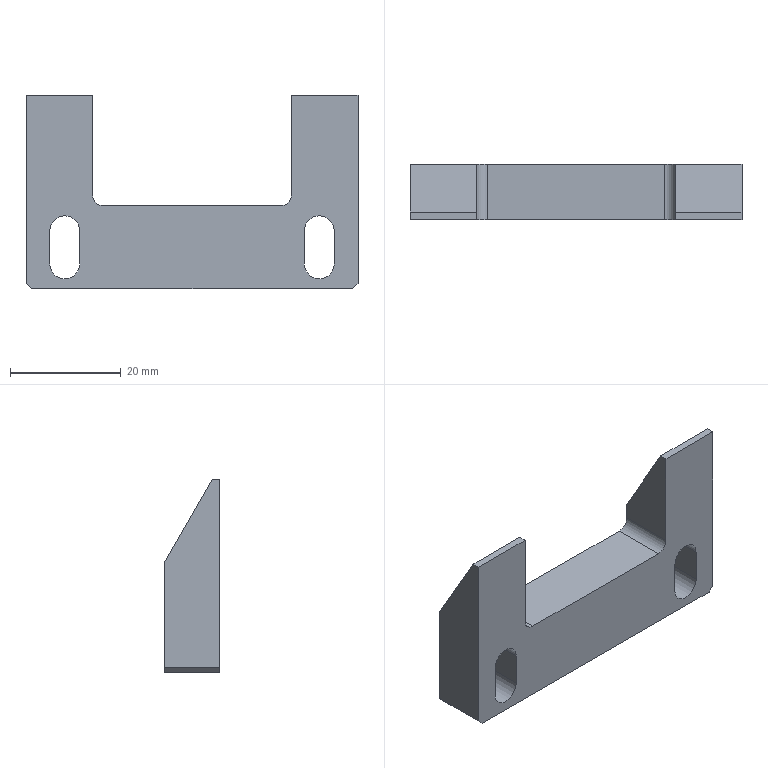Part | SolidWorks | features Chamfer 2, Cut 1, Extrusion 1, Fillet 1, ICE 1, MirrorPattern 1 | 1 solid | 26 faces | box 60 x 10 x 35 mm | volume 11142 mm3 | plane 18 | cylinder 8 | commonest cylinder face diameters 5.4 x6 4 x2
STEP:
#1=CARTESIAN_POINT('',(25.7,0.,-7.));
#2=VERTEX_POINT('',#1);
#3=CARTESIAN_POINT('',(23.,0.,-4.3));
#4=VERTEX_POINT('',#3);
#5=CARTESIAN_POINT('',(23.,0.,-7.));
#6=DIRECTION('',(0.,-1.,0.));
#7=DIRECTION('',(0.,0.,1.));
#8=AXIS2_PLACEMENT_3D('',#5,#6,#7);
#9=CIRCLE('',#8,2.7);
#10=EDGE_CURVE('',#2,#4,#9,.T.);
#11=ORIENTED_EDGE('',*,*,#10,.T.);
#12=CARTESIAN_POINT('',(23.,10.,-4.3));
#13=VERTEX_POINT('',#12);
#14=CARTESIAN_POINT('',(23.,0.,-4.3));
#15=DIRECTION('',(0.,1.,0.));
#16=VECTOR('',#15,1000.);
#17=LINE('',#14,#16);
#18=EDGE_CURVE('',#4,#13,#17,.T.);
#19=ORIENTED_EDGE('',*,*,#18,.T.);
#20=CARTESIAN_POINT('',(25.7,10.,-7.));
#21=VERTEX_POINT('',#20);
#22=CARTESIAN_POINT('',(23.,10.,-7.));
#23=DIRECTION('',(0.,-1.,0.));
#24=DIRECTION('',(0.,0.,1.));
#25=AXIS2_PLACEMENT_3D('',#22,#23,#24);
#26=CIRCLE('',#25,2.7);
#27=EDGE_CURVE('',#21,#13,#26,.T.);
#28=ORIENTED_EDGE('',*,*,#27,.F.);
#29=CARTESIAN_POINT('',(25.7,0.,-7.));
#30=DIRECTION('',(0.,1.,0.));
#31=VECTOR('',#30,1000.);
#32=LINE('',#29,#31);
#33=EDGE_CURVE('',#2,#21,#32,.T.);
#34=ORIENTED_EDGE('',*,*,#33,.F.);
#35=EDGE_LOOP('',(#11,#19,#28,#34));
#36=FACE_OUTER_BOUND('',#35,.T.);
#37=CARTESIAN_POINT('',(23.,0.,-7.));
#38=DIRECTION('',(0.,1.,0.));
#39=DIRECTION('',(0.,0.,1.));
#40=AXIS2_PLACEMENT_3D('',#37,#38,#39);
#41=CYLINDRICAL_SURFACE('',#40,2.7);
#42=ADVANCED_FACE('',(#36),#41,.F.);
#43=CARTESIAN_POINT('',(-23.,0.,-4.3));
#44=VERTEX_POINT('',#43);
#45=CARTESIAN_POINT('',(-20.3,0.,-7.));
#46=VERTEX_POINT('',#45);
#47=CARTESIAN_POINT('',(-23.,0.,-7.));
#48=DIRECTION('',(0.,1.,0.));
#49=DIRECTION('',(0.,0.,1.));
#50=AXIS2_PLACEMENT_3D('',#47,#48,#49);
#51=CIRCLE('',#50,2.7);
#52=EDGE_CURVE('',#44,#46,#51,.T.);
#53=ORIENTED_EDGE('',*,*,#52,.F.);
#54=CARTESIAN_POINT('',(-23.,10.,-4.3));
#55=VERTEX_POINT('',#54);
#56=CARTESIAN_POINT('',(-23.,0.,-4.3));
#57=DIRECTION('',(0.,1.,0.));
#58=VECTOR('',#57,1000.);
#59=LINE('',#56,#58);
#60=EDGE_CURVE('',#44,#55,#59,.T.);
#61=ORIENTED_EDGE('',*,*,#60,.T.);
#62=CARTESIAN_POINT('',(-20.3,10.,-7.));
#63=VERTEX_POINT('',#62);
#64=CARTESIAN_POINT('',(-23.,10.,-7.));
#65=DIRECTION('',(0.,1.,0.));
#66=DIRECTION('',(0.,0.,1.));
#67=AXIS2_PLACEMENT_3D('',#64,#65,#66);
#68=CIRCLE('',#67,2.7);
#69=EDGE_CURVE('',#55,#63,#68,.T.);
#70=ORIENTED_EDGE('',*,*,#69,.T.);
#71=CARTESIAN_POINT('',(-20.3,0.,-7.));
#72=DIRECTION('',(0.,1.,0.));
#73=VECTOR('',#72,1000.);
#74=LINE('',#71,#73);
#75=EDGE_CURVE('',#46,#63,#74,.T.);
#76=ORIENTED_EDGE('',*,*,#75,.F.);
#77=EDGE_LOOP('',(#53,#61,#70,#76));
#78=FACE_OUTER_BOUND('',#77,.T.);
#79=CARTESIAN_POINT('',(-23.,0.,-7.));
#80=DIRECTION('',(0.,1.,0.));
#81=DIRECTION('',(0.,0.,1.));
#82=AXIS2_PLACEMENT_3D('',#79,#80,#81);
#83=CYLINDRICAL_SURFACE('',#82,2.7);
#84=ADVANCED_FACE('',(#78),#83,.F.);
#85=CARTESIAN_POINT('',(30.,10.,2.5));
#86=VERTEX_POINT('',#85);
#87=CARTESIAN_POINT('',(30.,10.,-16.5));
#88=VERTEX_POINT('',#87);
#89=CARTESIAN_POINT('',(30.,10.,-17.5));
#90=DIRECTION('',(0.,0.,-1.));
#91=VECTOR('',#90,1000.);
#92=LINE('',#89,#91);
#93=EDGE_CURVE('',#86,#88,#92,.T.);
#94=ORIENTED_EDGE('',*,*,#93,.T.);
#95=CARTESIAN_POINT('',(29.,10.,-17.5));
#96=VERTEX_POINT('',#95);
#97=CARTESIAN_POINT('',(23.25,10.,-23.25));
#98=DIRECTION('',(-0.7071,0.,-0.7071));
#99=VECTOR('',#98,1000.);
#100=LINE('',#97,#99);
#101=EDGE_CURVE('',#88,#96,#100,.T.);
#102=ORIENTED_EDGE('',*,*,#101,.T.);
#103=CARTESIAN_POINT('',(-29.,10.,-17.5));
#104=VERTEX_POINT('',#103);
#105=CARTESIAN_POINT('',(-30.,10.,-17.5));
#106=DIRECTION('',(-1.,0.,0.));
#107=VECTOR('',#106,1000.);
#108=LINE('',#105,#107);
#109=EDGE_CURVE('',#96,#104,#108,.T.);
#110=ORIENTED_EDGE('',*,*,#109,.T.);
#111=CARTESIAN_POINT('',(-30.,10.,-16.5));
#112=VERTEX_POINT('',#111);
#113=CARTESIAN_POINT('',(-23.25,10.,-23.25));
#114=DIRECTION('',(-0.7071,0.,0.7071));
#115=VECTOR('',#114,1000.);
#116=LINE('',#113,#115);
#117=EDGE_CURVE('',#104,#112,#116,.T.);
#118=ORIENTED_EDGE('',*,*,#117,.T.);
#119=CARTESIAN_POINT('',(-30.,10.,2.5));
#120=VERTEX_POINT('',#119);
#121=CARTESIAN_POINT('',(-30.,10.,-17.5));
#122=DIRECTION('',(0.,0.,1.));
#123=VECTOR('',#122,1000.);
#124=LINE('',#121,#123);
#125=EDGE_CURVE('',#112,#120,#124,.T.);
#126=ORIENTED_EDGE('',*,*,#125,.T.);
#127=CARTESIAN_POINT('',(-18.,10.,2.5));
#128=VERTEX_POINT('',#127);
#129=CARTESIAN_POINT('',(30.,10.,2.5));
#130=DIRECTION('',(1.,0.,0.));
#131=VECTOR('',#130,1000.);
#132=LINE('',#129,#131);
#133=EDGE_CURVE('',#120,#128,#132,.T.);
#134=ORIENTED_EDGE('',*,*,#133,.T.);
#135=CARTESIAN_POINT('',(-18.,10.,-0.5));
#136=VERTEX_POINT('',#135);
#137=CARTESIAN_POINT('',(-18.,10.,17.5));
#138=DIRECTION('',(0.,0.,1.));
#139=VECTOR('',#138,1000.);
#140=LINE('',#137,#139);
#141=EDGE_CURVE('',#136,#128,#140,.T.);
#142=ORIENTED_EDGE('',*,*,#141,.F.);
#143=CARTESIAN_POINT('',(-16.,10.,-2.5));
#144=VERTEX_POINT('',#143);
#145=CARTESIAN_POINT('',(-16.,10.,-0.5));
#146=DIRECTION('',(0.,-1.,0.));
#147=DIRECTION('',(0.,0.,1.));
#148=AXIS2_PLACEMENT_3D('',#145,#146,#147);
#149=CIRCLE('',#148,2.);
#150=EDGE_CURVE('',#136,#144,#149,.T.);
#151=ORIENTED_EDGE('',*,*,#150,.T.);
#152=CARTESIAN_POINT('',(16.,10.,-2.5));
#153=VERTEX_POINT('',#152);
#154=CARTESIAN_POINT('',(-18.,10.,-2.5));
#155=DIRECTION('',(-1.,0.,0.));
#156=VECTOR('',#155,1000.);
#157=LINE('',#154,#156);
#158=EDGE_CURVE('',#153,#144,#157,.T.);
#159=ORIENTED_EDGE('',*,*,#158,.F.);
#160=CARTESIAN_POINT('',(18.,10.,-0.5));
#161=VERTEX_POINT('',#160);
#162=CARTESIAN_POINT('',(16.,10.,-0.5));
#163=DIRECTION('',(0.,-1.,0.));
#164=DIRECTION('',(0.,0.,1.));
#165=AXIS2_PLACEMENT_3D('',#162,#163,#164);
#166=CIRCLE('',#165,2.);
#167=EDGE_CURVE('',#153,#161,#166,.T.);
#168=ORIENTED_EDGE('',*,*,#167,.T.);
#169=CARTESIAN_POINT('',(18.,10.,2.5));
#170=VERTEX_POINT('',#169);
#171=CARTESIAN_POINT('',(18.,10.,17.5));
#172=DIRECTION('',(0.,0.,-1.));
#173=VECTOR('',#172,1000.);
#174=LINE('',#171,#173);
#175=EDGE_CURVE('',#170,#161,#174,.T.);
#176=ORIENTED_EDGE('',*,*,#175,.F.);
#177=CARTESIAN_POINT('',(30.,10.,2.5));
#178=DIRECTION('',(1.,0.,0.));
#179=VECTOR('',#178,1000.);
#180=LINE('',#177,#179);
#181=EDGE_CURVE('',#170,#86,#180,.T.);
#182=ORIENTED_EDGE('',*,*,#181,.T.);
#183=EDGE_LOOP('',(#94,#102,#110,#118,#126,#134,#142,#151,#159,#168,#176,#182));
#184=FACE_OUTER_BOUND('',#183,.T.);
#185=CARTESIAN_POINT('',(-20.3,10.,-13.));
#186=VERTEX_POINT('',#185);
#187=CARTESIAN_POINT('',(-25.7,10.,-13.));
#188=VERTEX_POINT('',#187);
#189=CARTESIAN_POINT('',(-23.,10.,-13.));
#190=DIRECTION('',(0.,1.,0.));
#191=DIRECTION('',(0.,0.,1.));
#192=AXIS2_PLACEMENT_3D('',#189,#190,#191);
#193=CIRCLE('',#192,2.7);
#194=EDGE_CURVE('',#186,#188,#193,.T.);
#195=ORIENTED_EDGE('',*,*,#194,.F.);
#196=CARTESIAN_POINT('',(-20.3,10.,-13.));
#197=DIRECTION('',(0.,0.,-1.));
#198=VECTOR('',#197,1000.);
#199=LINE('',#196,#198);
#200=EDGE_CURVE('',#63,#186,#199,.T.);
#201=ORIENTED_EDGE('',*,*,#200,.F.);
#202=ORIENTED_EDGE('',*,*,#69,.F.);
#203=CARTESIAN_POINT('',(-25.7,10.,-7.));
#204=VERTEX_POINT('',#203);
#205=CARTESIAN_POINT('',(-23.,10.,-7.));
#206=DIRECTION('',(0.,1.,0.));
#207=DIRECTION('',(0.,0.,1.));
#208=AXIS2_PLACEMENT_3D('',#205,#206,#207);
#209=CIRCLE('',#208,2.7);
#210=EDGE_CURVE('',#204,#55,#209,.T.);
#211=ORIENTED_EDGE('',*,*,#210,.F.);
#212=CARTESIAN_POINT('',(-25.7,10.,-13.));
#213=DIRECTION('',(0.,0.,1.));
#214=VECTOR('',#213,1000.);
#215=LINE('',#212,#214);
#216=EDGE_CURVE('',#188,#204,#215,.T.);
#217=ORIENTED_EDGE('',*,*,#216,.F.);
#218=EDGE_LOOP('',(#195,#201,#202,#211,#217));
#219=FACE_BOUND('',#218,.T.);
#220=CARTESIAN_POINT('',(20.3,10.,-7.));
#221=VERTEX_POINT('',#220);
#222=CARTESIAN_POINT('',(20.3,10.,-13.));
#223=VERTEX_POINT('',#222);
#224=CARTESIAN_POINT('',(20.3,10.,-13.));
#225=DIRECTION('',(0.,0.,-1.));
#226=VECTOR('',#225,1000.);
#227=LINE('',#224,#226);
#228=EDGE_CURVE('',#221,#223,#227,.T.);
#229=ORIENTED_EDGE('',*,*,#228,.T.);
#230=CARTESIAN_POINT('',(25.7,10.,-13.));
#231=VERTEX_POINT('',#230);
#232=CARTESIAN_POINT('',(23.,10.,-13.));
#233=DIRECTION('',(0.,-1.,0.));
#234=DIRECTION('',(0.,0.,1.));
#235=AXIS2_PLACEMENT_3D('',#232,#233,#234);
#236=CIRCLE('',#235,2.7);
#237=EDGE_CURVE('',#223,#231,#236,.T.);
#238=ORIENTED_EDGE('',*,*,#237,.T.);
#239=CARTESIAN_POINT('',(25.7,10.,-13.));
#240=DIRECTION('',(0.,0.,1.));
#241=VECTOR('',#240,1000.);
#242=LINE('',#239,#241);
#243=EDGE_CURVE('',#231,#21,#242,.T.);
#244=ORIENTED_EDGE('',*,*,#243,.T.);
#245=ORIENTED_EDGE('',*,*,#27,.T.);
#246=CARTESIAN_POINT('',(23.,10.,-7.));
#247=DIRECTION('',(0.,-1.,0.));
#248=DIRECTION('',(0.,0.,1.));
#249=AXIS2_PLACEMENT_3D('',#246,#247,#248);
#250=CIRCLE('',#249,2.7);
#251=EDGE_CURVE('',#13,#221,#250,.T.);
#252=ORIENTED_EDGE('',*,*,#251,.T.);
#253=EDGE_LOOP('',(#229,#238,#244,#245,#252));
#254=FACE_BOUND('',#253,.T.);
#255=CARTESIAN_POINT('',(0.,10.,0.));
#256=DIRECTION('',(0.,1.,0.));
#257=DIRECTION('',(0.,0.,1.));
#258=AXIS2_PLACEMENT_3D('',#255,#256,#257);
#259=PLANE('',#258);
#260=ADVANCED_FACE('',(#184,#219,#254),#259,.T.);
#261=CARTESIAN_POINT('',(29.,0.,-17.5));
#262=VERTEX_POINT('',#261);
#263=CARTESIAN_POINT('',(-29.,0.,-17.5));
#264=VERTEX_POINT('',#263);
#265=CARTESIAN_POINT('',(-30.,0.,-17.5));
#266=DIRECTION('',(-1.,0.,0.));
#267=VECTOR('',#266,1000.);
#268=LINE('',#265,#267);
#269=EDGE_CURVE('',#262,#264,#268,.T.);
#270=ORIENTED_EDGE('',*,*,#269,.F.);
#271=CARTESIAN_POINT('',(30.,0.,-16.5));
#272=VERTEX_POINT('',#271);
#273=CARTESIAN_POINT('',(29.,0.,-17.5));
#274=DIRECTION('',(0.7071,0.,0.7071));
#275=VECTOR('',#274,1000.);
#276=LINE('',#273,#275);
#277=EDGE_CURVE('',#262,#272,#276,.T.);
#278=ORIENTED_EDGE('',*,*,#277,.T.);
#279=CARTESIAN_POINT('',(30.,0.,17.5));
#280=VERTEX_POINT('',#279);
#281=CARTESIAN_POINT('',(30.,0.,-17.5));
#282=DIRECTION('',(0.,0.,-1.));
#283=VECTOR('',#282,1000.);
#284=LINE('',#281,#283);
#285=EDGE_CURVE('',#280,#272,#284,.T.);
#286=ORIENTED_EDGE('',*,*,#285,.F.);
#287=CARTESIAN_POINT('',(18.,0.,17.5));
#288=VERTEX_POINT('',#287);
#289=CARTESIAN_POINT('',(-30.,0.,17.5));
#290=DIRECTION('',(1.,0.,0.));
#291=VECTOR('',#290,1000.);
#292=LINE('',#289,#291);
#293=EDGE_CURVE('',#288,#280,#292,.T.);
#294=ORIENTED_EDGE('',*,*,#293,.F.);
#295=CARTESIAN_POINT('',(18.,0.,-0.5));
#296=VERTEX_POINT('',#295);
#297=CARTESIAN_POINT('',(18.,0.,17.5));
#298=DIRECTION('',(0.,0.,-1.));
#299=VECTOR('',#298,1000.);
#300=LINE('',#297,#299);
#301=EDGE_CURVE('',#288,#296,#300,.T.);
#302=ORIENTED_EDGE('',*,*,#301,.T.);
#303=CARTESIAN_POINT('',(16.,0.,-2.5));
#304=VERTEX_POINT('',#303);
#305=CARTESIAN_POINT('',(16.,0.,-0.5));
#306=DIRECTION('',(0.,1.,0.));
#307=DIRECTION('',(0.,0.,1.));
#308=AXIS2_PLACEMENT_3D('',#305,#306,#307);
#309=CIRCLE('',#308,2.);
#310=EDGE_CURVE('',#296,#304,#309,.T.);
#311=ORIENTED_EDGE('',*,*,#310,.T.);
#312=CARTESIAN_POINT('',(-16.,0.,-2.5));
#313=VERTEX_POINT('',#312);
#314=CARTESIAN_POINT('',(-18.,0.,-2.5));
#315=DIRECTION('',(-1.,0.,0.));
#316=VECTOR('',#315,1000.);
#317=LINE('',#314,#316);
#318=EDGE_CURVE('',#304,#313,#317,.T.);
#319=ORIENTED_EDGE('',*,*,#318,.T.);
#320=CARTESIAN_POINT('',(-18.,0.,-0.5));
#321=VERTEX_POINT('',#320);
#322=CARTESIAN_POINT('',(-16.,0.,-0.5));
#323=DIRECTION('',(0.,1.,0.));
#324=DIRECTION('',(0.,0.,1.));
#325=AXIS2_PLACEMENT_3D('',#322,#323,#324);
#326=CIRCLE('',#325,2.);
#327=EDGE_CURVE('',#313,#321,#326,.T.);
#328=ORIENTED_EDGE('',*,*,#327,.T.);
#329=CARTESIAN_POINT('',(-18.,0.,17.5));
#330=VERTEX_POINT('',#329);
#331=CARTESIAN_POINT('',(-18.,0.,17.5));
#332=DIRECTION('',(0.,0.,1.));
#333=VECTOR('',#332,1000.);
#334=LINE('',#331,#333);
#335=EDGE_CURVE('',#321,#330,#334,.T.);
#336=ORIENTED_EDGE('',*,*,#335,.T.);
#337=CARTESIAN_POINT('',(-30.,0.,17.5));
#338=VERTEX_POINT('',#337);
#339=CARTESIAN_POINT('',(-30.,0.,17.5));
#340=DIRECTION('',(1.,0.,0.));
#341=VECTOR('',#340,1000.);
#342=LINE('',#339,#341);
#343=EDGE_CURVE('',#338,#330,#342,.T.);
#344=ORIENTED_EDGE('',*,*,#343,.F.);
#345=CARTESIAN_POINT('',(-30.,0.,-16.5));
#346=VERTEX_POINT('',#345);
#347=CARTESIAN_POINT('',(-30.,0.,-17.5));
#348=DIRECTION('',(0.,0.,1.));
#349=VECTOR('',#348,1000.);
#350=LINE('',#347,#349);
#351=EDGE_CURVE('',#346,#338,#350,.T.);
#352=ORIENTED_EDGE('',*,*,#351,.F.);
#353=CARTESIAN_POINT('',(-30.,0.,-16.5));
#354=DIRECTION('',(0.7071,0.,-0.7071));
#355=VECTOR('',#354,1000.);
#356=LINE('',#353,#355);
#357=EDGE_CURVE('',#346,#264,#356,.T.);
#358=ORIENTED_EDGE('',*,*,#357,.T.);
#359=EDGE_LOOP('',(#270,#278,#286,#294,#302,#311,#319,#328,#336,#344,#352,#358));
#360=FACE_OUTER_BOUND('',#359,.T.);
#361=CARTESIAN_POINT('',(-20.3,0.,-13.));
#362=VERTEX_POINT('',#361);
#363=CARTESIAN_POINT('',(-20.3,0.,-13.));
#364=DIRECTION('',(0.,0.,-1.));
#365=VECTOR('',#364,1000.);
#366=LINE('',#363,#365);
#367=EDGE_CURVE('',#46,#362,#366,.T.);
#368=ORIENTED_EDGE('',*,*,#367,.T.);
#369=CARTESIAN_POINT('',(-25.7,0.,-13.));
#370=VERTEX_POINT('',#369);
#371=CARTESIAN_POINT('',(-23.,0.,-13.));
#372=DIRECTION('',(0.,1.,0.));
#373=DIRECTION('',(0.,0.,1.));
#374=AXIS2_PLACEMENT_3D('',#371,#372,#373);
#375=CIRCLE('',#374,2.7);
#376=EDGE_CURVE('',#362,#370,#375,.T.);
#377=ORIENTED_EDGE('',*,*,#376,.T.);
#378=CARTESIAN_POINT('',(-25.7,0.,-7.));
#379=VERTEX_POINT('',#378);
#380=CARTESIAN_POINT('',(-25.7,0.,-13.));
#381=DIRECTION('',(0.,0.,1.));
#382=VECTOR('',#381,1000.);
#383=LINE('',#380,#382);
#384=EDGE_CURVE('',#370,#379,#383,.T.);
#385=ORIENTED_EDGE('',*,*,#384,.T.);
#386=CARTESIAN_POINT('',(-23.,0.,-7.));
#387=DIRECTION('',(0.,1.,0.));
#388=DIRECTION('',(0.,0.,1.));
#389=AXIS2_PLACEMENT_3D('',#386,#387,#388);
#390=CIRCLE('',#389,2.7);
#391=EDGE_CURVE('',#379,#44,#390,.T.);
#392=ORIENTED_EDGE('',*,*,#391,.T.);
#393=ORIENTED_EDGE('',*,*,#52,.T.);
#394=EDGE_LOOP('',(#368,#377,#385,#392,#393));
#395=FACE_BOUND('',#394,.T.);
#396=CARTESIAN_POINT('',(20.3,0.,-13.));
#397=VERTEX_POINT('',#396);
#398=CARTESIAN_POINT('',(25.7,0.,-13.));
#399=VERTEX_POINT('',#398);
#400=CARTESIAN_POINT('',(23.,0.,-13.));
#401=DIRECTION('',(0.,-1.,0.));
#402=DIRECTION('',(0.,0.,1.));
#403=AXIS2_PLACEMENT_3D('',#400,#401,#402);
#404=CIRCLE('',#403,2.7);
#405=EDGE_CURVE('',#397,#399,#404,.T.);
#406=ORIENTED_EDGE('',*,*,#405,.F.);
#407=CARTESIAN_POINT('',(20.3,0.,-7.));
#408=VERTEX_POINT('',#407);
#409=CARTESIAN_POINT('',(20.3,0.,-13.));
#410=DIRECTION('',(0.,0.,-1.));
#411=VECTOR('',#410,1000.);
#412=LINE('',#409,#411);
#413=EDGE_CURVE('',#408,#397,#412,.T.);
#414=ORIENTED_EDGE('',*,*,#413,.F.);
#415=CARTESIAN_POINT('',(23.,0.,-7.));
#416=DIRECTION('',(0.,-1.,0.));
#417=DIRECTION('',(0.,0.,1.));
#418=AXIS2_PLACEMENT_3D('',#415,#416,#417);
#419=CIRCLE('',#418,2.7);
#420=EDGE_CURVE('',#4,#408,#419,.T.);
#421=ORIENTED_EDGE('',*,*,#420,.F.);
#422=ORIENTED_EDGE('',*,*,#10,.F.);
#423=CARTESIAN_POINT('',(25.7,0.,-13.));
#424=DIRECTION('',(0.,0.,1.));
#425=VECTOR('',#424,1000.);
#426=LINE('',#423,#425);
#427=EDGE_CURVE('',#399,#2,#426,.T.);
#428=ORIENTED_EDGE('',*,*,#427,.F.);
#429=EDGE_LOOP('',(#406,#414,#421,#422,#428));
#430=FACE_BOUND('',#429,.T.);
#431=CARTESIAN_POINT('',(0.,0.,0.));
#432=DIRECTION('',(0.,1.,0.));
#433=DIRECTION('',(0.,0.,1.));
#434=AXIS2_PLACEMENT_3D('',#431,#432,#433);
#435=PLANE('',#434);
#436=ADVANCED_FACE('',(#360,#395,#430),#435,.F.);
#437=ORIENTED_EDGE('',*,*,#343,.T.);
#438=CARTESIAN_POINT('',(-18.,1.34,17.5));
#439=VERTEX_POINT('',#438);
#440=CARTESIAN_POINT('',(-18.,0.,17.5));
#441=DIRECTION('',(0.,1.,0.));
#442=VECTOR('',#441,1000.);
#443=LINE('',#440,#442);
#444=EDGE_CURVE('',#330,#439,#443,.T.);
#445=ORIENTED_EDGE('',*,*,#444,.T.);
#446=CARTESIAN_POINT('',(-30.,1.34,17.5));
#447=VERTEX_POINT('',#446);
#448=CARTESIAN_POINT('',(-30.,1.34,17.5));
#449=DIRECTION('',(-1.,0.,0.));
#450=VECTOR('',#449,1000.);
#451=LINE('',#448,#450);
#452=EDGE_CURVE('',#439,#447,#451,.T.);
#453=ORIENTED_EDGE('',*,*,#452,.T.);
#454=CARTESIAN_POINT('',(-30.,10.,17.5));
#455=DIRECTION('',(0.,-1.,0.));
#456=VECTOR('',#455,1000.);
#457=LINE('',#454,#456);
#458=EDGE_CURVE('',#447,#338,#457,.T.);
#459=ORIENTED_EDGE('',*,*,#458,.T.);
#460=EDGE_LOOP('',(#437,#445,#453,#459));
#461=FACE_OUTER_BOUND('',#460,.T.);
#462=CARTESIAN_POINT('',(-30.,10.,17.5));
#463=DIRECTION('',(0.,0.,-1.));
#464=DIRECTION('',(-1.,0.,0.));
#465=AXIS2_PLACEMENT_3D('',#462,#463,#464);
#466=PLANE('',#465);
#467=ADVANCED_FACE('',(#461),#466,.F.);
#468=CARTESIAN_POINT('',(-18.,10.,2.5));
#469=DIRECTION('',(0.,-0.5,0.866));
#470=VECTOR('',#469,1000.);
#471=LINE('',#468,#470);
#472=EDGE_CURVE('',#128,#439,#471,.T.);
#473=ORIENTED_EDGE('',*,*,#472,.F.);
#474=ORIENTED_EDGE('',*,*,#133,.F.);
#475=CARTESIAN_POINT('',(-30.,10.,2.5));
#476=DIRECTION('',(0.,0.5,-0.866));
#477=VECTOR('',#476,1000.);
#478=LINE('',#475,#477);
#479=EDGE_CURVE('',#447,#120,#478,.T.);
#480=ORIENTED_EDGE('',*,*,#479,.F.);
#481=ORIENTED_EDGE('',*,*,#452,.F.);
#482=EDGE_LOOP('',(#473,#474,#480,#481));
#483=FACE_OUTER_BOUND('',#482,.T.);
#484=CARTESIAN_POINT('',(0.,10.,2.5));
#485=DIRECTION('',(0.,0.866,0.5));
#486=DIRECTION('',(-1.,0.,0.));
#487=AXIS2_PLACEMENT_3D('',#484,#485,#486);
#488=PLANE('',#487);
#489=ADVANCED_FACE('',(#483),#488,.T.);
#490=ORIENTED_EDGE('',*,*,#285,.T.);
#491=CARTESIAN_POINT('',(30.,10.,-16.5));
#492=DIRECTION('',(0.,1.,0.));
#493=VECTOR('',#492,1000.);
#494=LINE('',#491,#493);
#495=EDGE_CURVE('',#272,#88,#494,.T.);
#496=ORIENTED_EDGE('',*,*,#495,.T.);
#497=ORIENTED_EDGE('',*,*,#93,.F.);
#498=CARTESIAN_POINT('',(30.,1.34,17.5));
#499=VERTEX_POINT('',#498);
#500=CARTESIAN_POINT('',(30.,10.,2.5));
#501=DIRECTION('',(0.,-0.5,0.866));
#502=VECTOR('',#501,1000.);
#503=LINE('',#500,#502);
#504=EDGE_CURVE('',#86,#499,#503,.T.);
#505=ORIENTED_EDGE('',*,*,#504,.T.);
#506=CARTESIAN_POINT('',(30.,10.,17.5));
#507=DIRECTION('',(0.,-1.,0.));
#508=VECTOR('',#507,1000.);
#509=LINE('',#506,#508);
#510=EDGE_CURVE('',#499,#280,#509,.T.);
#511=ORIENTED_EDGE('',*,*,#510,.T.);
#512=EDGE_LOOP('',(#490,#496,#497,#505,#511));
#513=FACE_OUTER_BOUND('',#512,.T.);
#514=CARTESIAN_POINT('',(30.,10.,-17.5));
#515=DIRECTION('',(-1.,0.,0.));
#516=DIRECTION('',(0.,0.,1.));
#517=AXIS2_PLACEMENT_3D('',#514,#515,#516);
#518=PLANE('',#517);
#519=ADVANCED_FACE('',(#513),#518,.F.);
#520=ORIENTED_EDGE('',*,*,#109,.F.);
#521=CARTESIAN_POINT('',(29.,10.,-17.5));
#522=DIRECTION('',(0.,-1.,0.));
#523=VECTOR('',#522,1000.);
#524=LINE('',#521,#523);
#525=EDGE_CURVE('',#96,#262,#524,.T.);
#526=ORIENTED_EDGE('',*,*,#525,.T.);
#527=ORIENTED_EDGE('',*,*,#269,.T.);
#528=CARTESIAN_POINT('',(-29.,10.,-17.5));
#529=DIRECTION('',(0.,1.,0.));
#530=VECTOR('',#529,1000.);
#531=LINE('',#528,#530);
#532=EDGE_CURVE('',#264,#104,#531,.T.);
#533=ORIENTED_EDGE('',*,*,#532,.T.);
#534=EDGE_LOOP('',(#520,#526,#527,#533));
#535=FACE_OUTER_BOUND('',#534,.T.);
#536=CARTESIAN_POINT('',(-30.,10.,-17.5));
#537=DIRECTION('',(0.,0.,1.));
#538=DIRECTION('',(1.,0.,0.));
#539=AXIS2_PLACEMENT_3D('',#536,#537,#538);
#540=PLANE('',#539);
#541=ADVANCED_FACE('',(#535),#540,.F.);
#542=ORIENTED_EDGE('',*,*,#125,.F.);
#543=CARTESIAN_POINT('',(-30.,10.,-16.5));
#544=DIRECTION('',(0.,-1.,0.));
#545=VECTOR('',#544,1000.);
#546=LINE('',#543,#545);
#547=EDGE_CURVE('',#112,#346,#546,.T.);
#548=ORIENTED_EDGE('',*,*,#547,.T.);
#549=ORIENTED_EDGE('',*,*,#351,.T.);
#550=ORIENTED_EDGE('',*,*,#458,.F.);
#551=ORIENTED_EDGE('',*,*,#479,.T.);
#552=EDGE_LOOP('',(#542,#548,#549,#550,#551));
#553=FACE_OUTER_BOUND('',#552,.T.);
#554=CARTESIAN_POINT('',(-30.,10.,-17.5));
#555=DIRECTION('',(1.,0.,0.));
#556=DIRECTION('',(0.,0.,-1.));
#557=AXIS2_PLACEMENT_3D('',#554,#555,#556);
#558=PLANE('',#557);
#559=ADVANCED_FACE('',(#553),#558,.F.);
#560=CARTESIAN_POINT('',(18.,1.34,17.5));
#561=VERTEX_POINT('',#560);
#562=CARTESIAN_POINT('',(-30.,1.34,17.5));
#563=DIRECTION('',(-1.,0.,0.));
#564=VECTOR('',#563,1000.);
#565=LINE('',#562,#564);
#566=EDGE_CURVE('',#499,#561,#565,.T.);
#567=ORIENTED_EDGE('',*,*,#566,.T.);
#568=CARTESIAN_POINT('',(18.,0.,17.5));
#569=DIRECTION('',(0.,1.,0.));
#570=VECTOR('',#569,1000.);
#571=LINE('',#568,#570);
#572=EDGE_CURVE('',#288,#561,#571,.T.);
#573=ORIENTED_EDGE('',*,*,#572,.F.);
#574=ORIENTED_EDGE('',*,*,#293,.T.);
#575=ORIENTED_EDGE('',*,*,#510,.F.);
#576=EDGE_LOOP('',(#567,#573,#574,#575));
#577=FACE_OUTER_BOUND('',#576,.T.);
#578=CARTESIAN_POINT('',(-30.,10.,17.5));
#579=DIRECTION('',(0.,0.,-1.));
#580=DIRECTION('',(-1.,0.,0.));
#581=AXIS2_PLACEMENT_3D('',#578,#579,#580);
#582=PLANE('',#581);
#583=ADVANCED_FACE('',(#577),#582,.F.);
#584=CARTESIAN_POINT('',(18.,10.,2.5));
#585=DIRECTION('',(0.,0.5,-0.866));
#586=VECTOR('',#585,1000.);
#587=LINE('',#584,#586);
#588=EDGE_CURVE('',#561,#170,#587,.T.);
#589=ORIENTED_EDGE('',*,*,#588,.F.);
#590=ORIENTED_EDGE('',*,*,#566,.F.);
#591=ORIENTED_EDGE('',*,*,#504,.F.);
#592=ORIENTED_EDGE('',*,*,#181,.F.);
#593=EDGE_LOOP('',(#589,#590,#591,#592));
#594=FACE_OUTER_BOUND('',#593,.T.);
#595=CARTESIAN_POINT('',(0.,10.,2.5));
#596=DIRECTION('',(0.,0.866,0.5));
#597=DIRECTION('',(-1.,0.,0.));
#598=AXIS2_PLACEMENT_3D('',#595,#596,#597);
#599=PLANE('',#598);
#600=ADVANCED_FACE('',(#594),#599,.T.);
#601=ORIENTED_EDGE('',*,*,#335,.F.);
#602=CARTESIAN_POINT('',(-18.,10.,-0.5));
#603=DIRECTION('',(0.,1.,0.));
#604=VECTOR('',#603,1000.);
#605=LINE('',#602,#604);
#606=EDGE_CURVE('',#321,#136,#605,.T.);
#607=ORIENTED_EDGE('',*,*,#606,.T.);
#608=ORIENTED_EDGE('',*,*,#141,.T.);
#609=ORIENTED_EDGE('',*,*,#472,.T.);
#610=ORIENTED_EDGE('',*,*,#444,.F.);
#611=EDGE_LOOP('',(#601,#607,#608,#609,#610));
#612=FACE_OUTER_BOUND('',#611,.T.);
#613=CARTESIAN_POINT('',(-18.,0.,17.5));
#614=DIRECTION('',(-1.,0.,0.));
#615=DIRECTION('',(0.,0.,1.));
#616=AXIS2_PLACEMENT_3D('',#613,#614,#615);
#617=PLANE('',#616);
#618=ADVANCED_FACE('',(#612),#617,.F.);
#619=ORIENTED_EDGE('',*,*,#318,.F.);
#620=CARTESIAN_POINT('',(16.,10.,-2.5));
#621=DIRECTION('',(0.,1.,0.));
#622=VECTOR('',#621,1000.);
#623=LINE('',#620,#622);
#624=EDGE_CURVE('',#304,#153,#623,.T.);
#625=ORIENTED_EDGE('',*,*,#624,.T.);
#626=ORIENTED_EDGE('',*,*,#158,.T.);
#627=CARTESIAN_POINT('',(-16.,0.,-2.5));
#628=DIRECTION('',(0.,-1.,0.));
#629=VECTOR('',#628,1000.);
#630=LINE('',#627,#629);
#631=EDGE_CURVE('',#144,#313,#630,.T.);
#632=ORIENTED_EDGE('',*,*,#631,.T.);
#633=EDGE_LOOP('',(#619,#625,#626,#632));
#634=FACE_OUTER_BOUND('',#633,.T.);
#635=CARTESIAN_POINT('',(-18.,0.,-2.5));
#636=DIRECTION('',(0.,0.,-1.));
#637=DIRECTION('',(-1.,0.,0.));
#638=AXIS2_PLACEMENT_3D('',#635,#636,#637);
#639=PLANE('',#638);
#640=ADVANCED_FACE('',(#634),#639,.F.);
#641=ORIENTED_EDGE('',*,*,#175,.T.);
#642=CARTESIAN_POINT('',(18.,0.,-0.5));
#643=DIRECTION('',(0.,-1.,0.));
#644=VECTOR('',#643,1000.);
#645=LINE('',#642,#644);
#646=EDGE_CURVE('',#161,#296,#645,.T.);
#647=ORIENTED_EDGE('',*,*,#646,.T.);
#648=ORIENTED_EDGE('',*,*,#301,.F.);
#649=ORIENTED_EDGE('',*,*,#572,.T.);
#650=ORIENTED_EDGE('',*,*,#588,.T.);
#651=EDGE_LOOP('',(#641,#647,#648,#649,#650));
#652=FACE_OUTER_BOUND('',#651,.T.);
#653=CARTESIAN_POINT('',(18.,0.,17.5));
#654=DIRECTION('',(1.,0.,0.));
#655=DIRECTION('',(0.,0.,-1.));
#656=AXIS2_PLACEMENT_3D('',#653,#654,#655);
#657=PLANE('',#656);
#658=ADVANCED_FACE('',(#652),#657,.F.);
#659=ORIENTED_EDGE('',*,*,#310,.F.);
#660=ORIENTED_EDGE('',*,*,#646,.F.);
#661=ORIENTED_EDGE('',*,*,#167,.F.);
#662=ORIENTED_EDGE('',*,*,#624,.F.);
#663=EDGE_LOOP('',(#659,#660,#661,#662));
#664=FACE_OUTER_BOUND('',#663,.T.);
#665=CARTESIAN_POINT('',(16.,0.,-0.5));
#666=DIRECTION('',(0.,-1.,0.));
#667=DIRECTION('',(0.,0.,-1.));
#668=AXIS2_PLACEMENT_3D('',#665,#666,#667);
#669=CYLINDRICAL_SURFACE('',#668,2.);
#670=ADVANCED_FACE('',(#664),#669,.F.);
#671=ORIENTED_EDGE('',*,*,#327,.F.);
#672=ORIENTED_EDGE('',*,*,#631,.F.);
#673=ORIENTED_EDGE('',*,*,#150,.F.);
#674=ORIENTED_EDGE('',*,*,#606,.F.);
#675=EDGE_LOOP('',(#671,#672,#673,#674));
#676=FACE_OUTER_BOUND('',#675,.T.);
#677=CARTESIAN_POINT('',(-16.,0.,-0.5));
#678=DIRECTION('',(0.,-1.,0.));
#679=DIRECTION('',(0.,0.,-1.));
#680=AXIS2_PLACEMENT_3D('',#677,#678,#679);
#681=CYLINDRICAL_SURFACE('',#680,2.);
#682=ADVANCED_FACE('',(#676),#681,.F.);
#683=ORIENTED_EDGE('',*,*,#194,.T.);
#684=CARTESIAN_POINT('',(-25.7,0.,-13.));
#685=DIRECTION('',(0.,1.,0.));
#686=VECTOR('',#685,1000.);
#687=LINE('',#684,#686);
#688=EDGE_CURVE('',#370,#188,#687,.T.);
#689=ORIENTED_EDGE('',*,*,#688,.F.);
#690=ORIENTED_EDGE('',*,*,#376,.F.);
#691=CARTESIAN_POINT('',(-20.3,0.,-13.));
#692=DIRECTION('',(0.,1.,0.));
#693=VECTOR('',#692,1000.);
#694=LINE('',#691,#693);
#695=EDGE_CURVE('',#362,#186,#694,.T.);
#696=ORIENTED_EDGE('',*,*,#695,.T.);
#697=EDGE_LOOP('',(#683,#689,#690,#696));
#698=FACE_OUTER_BOUND('',#697,.T.);
#699=CARTESIAN_POINT('',(-23.,0.,-13.));
#700=DIRECTION('',(0.,1.,0.));
#701=DIRECTION('',(0.,0.,1.));
#702=AXIS2_PLACEMENT_3D('',#699,#700,#701);
#703=CYLINDRICAL_SURFACE('',#702,2.7);
#704=ADVANCED_FACE('',(#698),#703,.F.);
#705=ORIENTED_EDGE('',*,*,#200,.T.);
#706=ORIENTED_EDGE('',*,*,#695,.F.);
#707=ORIENTED_EDGE('',*,*,#367,.F.);
#708=ORIENTED_EDGE('',*,*,#75,.T.);
#709=EDGE_LOOP('',(#705,#706,#707,#708));
#710=FACE_OUTER_BOUND('',#709,.T.);
#711=CARTESIAN_POINT('',(-20.3,0.,-13.));
#712=DIRECTION('',(1.,0.,0.));
#713=DIRECTION('',(0.,0.,-1.));
#714=AXIS2_PLACEMENT_3D('',#711,#712,#713);
#715=PLANE('',#714);
#716=ADVANCED_FACE('',(#710),#715,.F.);
#717=ORIENTED_EDGE('',*,*,#60,.F.);
#718=ORIENTED_EDGE('',*,*,#391,.F.);
#719=CARTESIAN_POINT('',(-25.7,0.,-7.));
#720=DIRECTION('',(0.,1.,0.));
#721=VECTOR('',#720,1000.);
#722=LINE('',#719,#721);
#723=EDGE_CURVE('',#379,#204,#722,.T.);
#724=ORIENTED_EDGE('',*,*,#723,.T.);
#725=ORIENTED_EDGE('',*,*,#210,.T.);
#726=EDGE_LOOP('',(#717,#718,#724,#725));
#727=FACE_OUTER_BOUND('',#726,.T.);
#728=CARTESIAN_POINT('',(-23.,0.,-7.));
#729=DIRECTION('',(0.,1.,0.));
#730=DIRECTION('',(0.,0.,1.));
#731=AXIS2_PLACEMENT_3D('',#728,#729,#730);
#732=CYLINDRICAL_SURFACE('',#731,2.7);
#733=ADVANCED_FACE('',(#727),#732,.F.);
#734=ORIENTED_EDGE('',*,*,#216,.T.);
#735=ORIENTED_EDGE('',*,*,#723,.F.);
#736=ORIENTED_EDGE('',*,*,#384,.F.);
#737=ORIENTED_EDGE('',*,*,#688,.T.);
#738=EDGE_LOOP('',(#734,#735,#736,#737));
#739=FACE_OUTER_BOUND('',#738,.T.);
#740=CARTESIAN_POINT('',(-25.7,0.,-13.));
#741=DIRECTION('',(-1.,0.,0.));
#742=DIRECTION('',(0.,0.,1.));
#743=AXIS2_PLACEMENT_3D('',#740,#741,#742);
#744=PLANE('',#743);
#745=ADVANCED_FACE('',(#739),#744,.F.);
#746=ORIENTED_EDGE('',*,*,#237,.F.);
#747=CARTESIAN_POINT('',(20.3,0.,-13.));
#748=DIRECTION('',(0.,1.,0.));
#749=VECTOR('',#748,1000.);
#750=LINE('',#747,#749);
#751=EDGE_CURVE('',#397,#223,#750,.T.);
#752=ORIENTED_EDGE('',*,*,#751,.F.);
#753=ORIENTED_EDGE('',*,*,#405,.T.);
#754=CARTESIAN_POINT('',(25.7,0.,-13.));
#755=DIRECTION('',(0.,1.,0.));
#756=VECTOR('',#755,1000.);
#757=LINE('',#754,#756);
#758=EDGE_CURVE('',#399,#231,#757,.T.);
#759=ORIENTED_EDGE('',*,*,#758,.T.);
#760=EDGE_LOOP('',(#746,#752,#753,#759));
#761=FACE_OUTER_BOUND('',#760,.T.);
#762=CARTESIAN_POINT('',(23.,0.,-13.));
#763=DIRECTION('',(0.,1.,0.));
#764=DIRECTION('',(0.,0.,1.));
#765=AXIS2_PLACEMENT_3D('',#762,#763,#764);
#766=CYLINDRICAL_SURFACE('',#765,2.7);
#767=ADVANCED_FACE('',(#761),#766,.F.);
#768=ORIENTED_EDGE('',*,*,#243,.F.);
#769=ORIENTED_EDGE('',*,*,#758,.F.);
#770=ORIENTED_EDGE('',*,*,#427,.T.);
#771=ORIENTED_EDGE('',*,*,#33,.T.);
#772=EDGE_LOOP('',(#768,#769,#770,#771));
#773=FACE_OUTER_BOUND('',#772,.T.);
#774=CARTESIAN_POINT('',(25.7,0.,-13.));
#775=DIRECTION('',(-1.,0.,0.));
#776=DIRECTION('',(0.,0.,1.));
#777=AXIS2_PLACEMENT_3D('',#774,#775,#776);
#778=PLANE('',#777);
#779=ADVANCED_FACE('',(#773),#778,.T.);
#780=ORIENTED_EDGE('',*,*,#18,.F.);
#781=ORIENTED_EDGE('',*,*,#420,.T.);
#782=CARTESIAN_POINT('',(20.3,0.,-7.));
#783=DIRECTION('',(0.,1.,0.));
#784=VECTOR('',#783,1000.);
#785=LINE('',#782,#784);
#786=EDGE_CURVE('',#408,#221,#785,.T.);
#787=ORIENTED_EDGE('',*,*,#786,.T.);
#788=ORIENTED_EDGE('',*,*,#251,.F.);
#789=EDGE_LOOP('',(#780,#781,#787,#788));
#790=FACE_OUTER_BOUND('',#789,.T.);
#791=CARTESIAN_POINT('',(23.,0.,-7.));
#792=DIRECTION('',(0.,1.,0.));
#793=DIRECTION('',(0.,0.,1.));
#794=AXIS2_PLACEMENT_3D('',#791,#792,#793);
#795=CYLINDRICAL_SURFACE('',#794,2.7);
#796=ADVANCED_FACE('',(#790),#795,.F.);
#797=ORIENTED_EDGE('',*,*,#228,.F.);
#798=ORIENTED_EDGE('',*,*,#786,.F.);
#799=ORIENTED_EDGE('',*,*,#413,.T.);
#800=ORIENTED_EDGE('',*,*,#751,.T.);
#801=EDGE_LOOP('',(#797,#798,#799,#800));
#802=FACE_OUTER_BOUND('',#801,.T.);
#803=CARTESIAN_POINT('',(20.3,0.,-13.));
#804=DIRECTION('',(1.,0.,0.));
#805=DIRECTION('',(0.,0.,-1.));
#806=AXIS2_PLACEMENT_3D('',#803,#804,#805);
#807=PLANE('',#806);
#808=ADVANCED_FACE('',(#802),#807,.T.);
#809=ORIENTED_EDGE('',*,*,#101,.F.);
#810=ORIENTED_EDGE('',*,*,#495,.F.);
#811=ORIENTED_EDGE('',*,*,#277,.F.);
#812=ORIENTED_EDGE('',*,*,#525,.F.);
#813=EDGE_LOOP('',(#809,#810,#811,#812));
#814=FACE_OUTER_BOUND('',#813,.T.);
#815=CARTESIAN_POINT('',(29.,10.,-17.5));
#816=DIRECTION('',(-0.7071,0.,0.7071));
#817=DIRECTION('',(0.,-1.,0.));
#818=AXIS2_PLACEMENT_3D('',#815,#816,#817);
#819=PLANE('',#818);
#820=ADVANCED_FACE('',(#814),#819,.F.);
#821=ORIENTED_EDGE('',*,*,#117,.F.);
#822=ORIENTED_EDGE('',*,*,#532,.F.);
#823=ORIENTED_EDGE('',*,*,#357,.F.);
#824=ORIENTED_EDGE('',*,*,#547,.F.);
#825=EDGE_LOOP('',(#821,#822,#823,#824));
#826=FACE_OUTER_BOUND('',#825,.T.);
#827=CARTESIAN_POINT('',(-30.,10.,-16.5));
#828=DIRECTION('',(0.7071,0.,0.7071));
#829=DIRECTION('',(0.,-1.,0.));
#830=AXIS2_PLACEMENT_3D('',#827,#828,#829);
#831=PLANE('',#830);
#832=ADVANCED_FACE('',(#826),#831,.F.);
#833=CLOSED_SHELL('',(#42,#84,#260,#436,#467,#489,#519,#541,#559,#583,#600,#618,#640,#658,#670,#682,#704,#716,#733,#745,#767,#779,#796,#808,#820,#832));
#834=MANIFOLD_SOLID_BREP('',#833);
#835=CARTESIAN_POINT('',(0.,0.,0.));
#836=DIRECTION('',(0.,0.,1.));
#837=DIRECTION('',(1.,0.,0.));
#838=AXIS2_PLACEMENT_3D('',#835,#836,#837);
#839=(LENGTH_UNIT()NAMED_UNIT(*)SI_UNIT(.MILLI.,.METRE.));
#840=UNCERTAINTY_MEASURE_WITH_UNIT(LENGTH_MEASURE(0.00001),#839,'','');
#841=(NAMED_UNIT(*)PLANE_ANGLE_UNIT()SI_UNIT($,.RADIAN.));
#842=(NAMED_UNIT(*)SI_UNIT($,.STERADIAN.)SOLID_ANGLE_UNIT());
#843=(GEOMETRIC_REPRESENTATION_CONTEXT(3)GLOBAL_UNCERTAINTY_ASSIGNED_CONTEXT((#840))GLOBAL_UNIT_ASSIGNED_CONTEXT((#839,#841,#842))REPRESENTATION_CONTEXT('',''));
#844=ADVANCED_BREP_SHAPE_REPRESENTATION('',(#834,#838),#843);